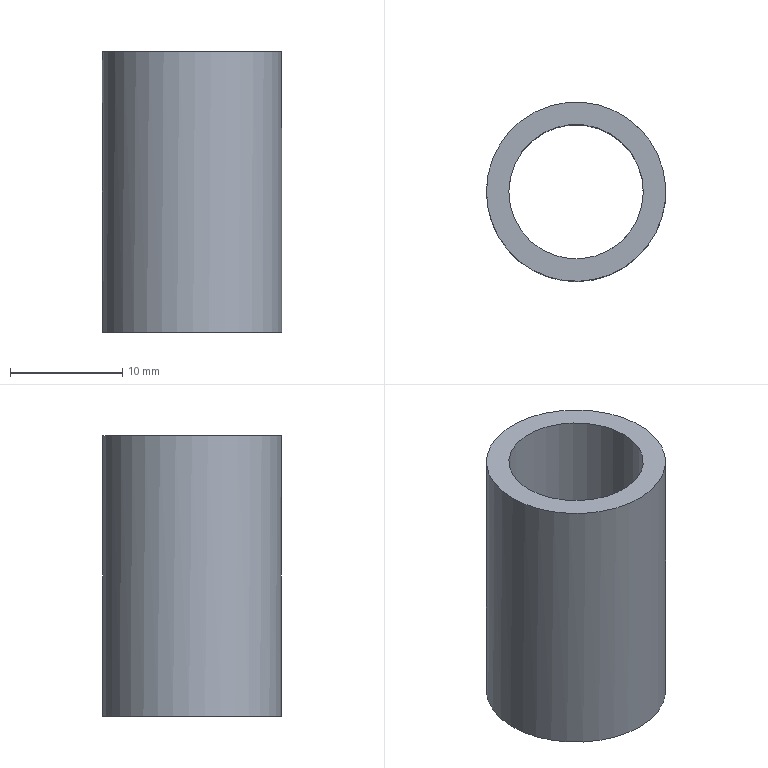Part | NX | features solid 2 | 1 solid | 4 faces | box 16 x 16 x 25 mm | volume 2199 mm3 | cylinder 2 | plane 2 | commonest cylinder face diameters 12 x1 16 x1
STEP:
#1=CARTESIAN_POINT('',(-232.777,185.339,-30.));
#2=VERTEX_POINT('',#1);
#3=CARTESIAN_POINT('',(-226.777,185.339,-30.));
#4=DIRECTION('',(0.,0.,-1.));
#5=DIRECTION('',(-1.,0.,0.));
#6=AXIS2_PLACEMENT_3D('',#3,#4,#5);
#7=CIRCLE('',#6,6.);
#8=EDGE_CURVE('',#2,#2,#7,.T.);
#9=ORIENTED_EDGE('',*,*,#8,.F.);
#10=EDGE_LOOP('',(#9));
#11=FACE_BOUND('',#10,.T.);
#12=CARTESIAN_POINT('',(-221.339,182.804,-55.));
#13=VERTEX_POINT('',#12);
#14=CARTESIAN_POINT('',(-226.777,185.339,-55.));
#15=DIRECTION('',(0.,0.,-1.));
#16=DIRECTION('',(0.9063,-0.4226,0.));
#17=AXIS2_PLACEMENT_3D('',#14,#15,#16);
#18=CIRCLE('',#17,6.);
#19=EDGE_CURVE('',#13,#13,#18,.F.);
#20=ORIENTED_EDGE('',*,*,#19,.F.);
#21=EDGE_LOOP('',(#20));
#22=FACE_BOUND('',#21,.T.);
#23=CARTESIAN_POINT('',(-226.777,185.339,-55.));
#24=DIRECTION('',(0.,0.,1.));
#25=DIRECTION('',(0.9063,-0.4226,0.));
#26=AXIS2_PLACEMENT_3D('',#23,#24,#25);
#27=CYLINDRICAL_SURFACE('',#26,6.);
#28=ADVANCED_FACE('',(#11,#22),#27,.F.);
#29=ORIENTED_EDGE('',*,*,#19,.T.);
#30=EDGE_LOOP('',(#29));
#31=FACE_BOUND('',#30,.T.);
#32=CARTESIAN_POINT('',(-223.396,192.59,-55.));
#33=VERTEX_POINT('',#32);
#34=CARTESIAN_POINT('',(-226.777,185.339,-55.));
#35=DIRECTION('',(0.,0.,1.));
#36=DIRECTION('',(0.4226,0.9063,0.));
#37=AXIS2_PLACEMENT_3D('',#34,#35,#36);
#38=CIRCLE('',#37,8.);
#39=EDGE_CURVE('',#33,#33,#38,.T.);
#40=ORIENTED_EDGE('',*,*,#39,.F.);
#41=EDGE_LOOP('',(#40));
#42=FACE_BOUND('',#41,.T.);
#43=CARTESIAN_POINT('',(-226.777,185.339,-55.));
#44=DIRECTION('',(0.,0.,1.));
#45=DIRECTION('',(0.9063,-0.4226,0.));
#46=AXIS2_PLACEMENT_3D('',#43,#44,#45);
#47=PLANE('',#46);
#48=ADVANCED_FACE('',(#31,#42),#47,.F.);
#49=CARTESIAN_POINT('',(-234.777,185.339,-30.));
#50=VERTEX_POINT('',#49);
#51=CARTESIAN_POINT('',(-226.777,185.339,-30.));
#52=DIRECTION('',(0.,0.,-1.));
#53=DIRECTION('',(-1.,0.,0.));
#54=AXIS2_PLACEMENT_3D('',#51,#52,#53);
#55=CIRCLE('',#54,8.);
#56=EDGE_CURVE('',#50,#50,#55,.T.);
#57=ORIENTED_EDGE('',*,*,#56,.T.);
#58=EDGE_LOOP('',(#57));
#59=FACE_BOUND('',#58,.T.);
#60=ORIENTED_EDGE('',*,*,#39,.T.);
#61=EDGE_LOOP('',(#60));
#62=FACE_BOUND('',#61,.T.);
#63=CARTESIAN_POINT('',(-226.777,185.339,-55.));
#64=DIRECTION('',(0.,0.,1.));
#65=DIRECTION('',(0.9063,-0.4226,0.));
#66=AXIS2_PLACEMENT_3D('',#63,#64,#65);
#67=CYLINDRICAL_SURFACE('',#66,8.);
#68=ADVANCED_FACE('',(#59,#62),#67,.T.);
#69=ORIENTED_EDGE('',*,*,#8,.T.);
#70=EDGE_LOOP('',(#69));
#71=FACE_BOUND('',#70,.T.);
#72=ORIENTED_EDGE('',*,*,#56,.F.);
#73=EDGE_LOOP('',(#72));
#74=FACE_BOUND('',#73,.T.);
#75=CARTESIAN_POINT('',(-315.526,-4.985,-30.));
#76=DIRECTION('',(0.,0.,-1.));
#77=DIRECTION('',(-1.,0.,0.));
#78=AXIS2_PLACEMENT_3D('',#75,#76,#77);
#79=PLANE('',#78);
#80=ADVANCED_FACE('',(#71,#74),#79,.F.);
#81=CLOSED_SHELL('',(#28,#48,#68,#80));
#82=MANIFOLD_SOLID_BREP('',#81);
#83=(LENGTH_UNIT()NAMED_UNIT(*)SI_UNIT(.MILLI.,.METRE.));
#84=UNCERTAINTY_MEASURE_WITH_UNIT(LENGTH_MEASURE(0.00001),#83,'','');
#85=(NAMED_UNIT(*)PLANE_ANGLE_UNIT()SI_UNIT($,.RADIAN.));
#86=(NAMED_UNIT(*)SI_UNIT($,.STERADIAN.)SOLID_ANGLE_UNIT());
#87=(GEOMETRIC_REPRESENTATION_CONTEXT(3)GLOBAL_UNCERTAINTY_ASSIGNED_CONTEXT((#84))GLOBAL_UNIT_ASSIGNED_CONTEXT((#83,#85,#86))REPRESENTATION_CONTEXT('',''));
#88=ADVANCED_BREP_SHAPE_REPRESENTATION('',(#82),#87);